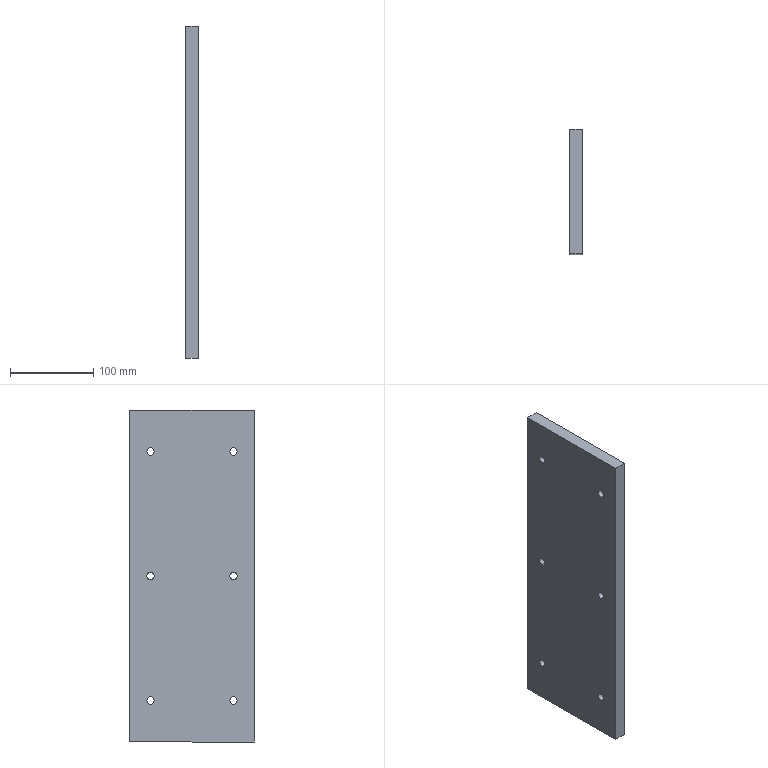Part | SolidWorks | features Extrusion 1, HoleWzd 1 | 1 solid | 36 faces | box 15 x 150 x 400 mm | volume 888167 mm3 | cylinder 24 | plane 12 | commonest cylinder face diameters 9 x12 15 x12
STEP:
#1=CARTESIAN_POINT('',(6.,50.,157.5));
#2=VERTEX_POINT('',#1);
#3=CARTESIAN_POINT('',(6.,50.,142.5));
#4=VERTEX_POINT('',#3);
#5=CARTESIAN_POINT('',(6.,50.,150.));
#6=DIRECTION('',(1.,0.,0.));
#7=DIRECTION('',(0.,0.,-1.));
#8=AXIS2_PLACEMENT_3D('',#5,#6,#7);
#9=CIRCLE('',#8,7.5);
#10=EDGE_CURVE('',#2,#4,#9,.T.);
#11=ORIENTED_EDGE('',*,*,#10,.F.);
#12=CARTESIAN_POINT('',(15.,50.,157.5));
#13=VERTEX_POINT('',#12);
#14=CARTESIAN_POINT('',(15.,50.,157.5));
#15=DIRECTION('',(1.,0.,0.));
#16=VECTOR('',#15,1000.);
#17=LINE('',#14,#16);
#18=EDGE_CURVE('',#2,#13,#17,.T.);
#19=ORIENTED_EDGE('',*,*,#18,.T.);
#20=CARTESIAN_POINT('',(15.,50.,142.5));
#21=VERTEX_POINT('',#20);
#22=CARTESIAN_POINT('',(15.,50.,150.));
#23=DIRECTION('',(1.,0.,0.));
#24=DIRECTION('',(0.,0.,-1.));
#25=AXIS2_PLACEMENT_3D('',#22,#23,#24);
#26=CIRCLE('',#25,7.5);
#27=EDGE_CURVE('',#13,#21,#26,.T.);
#28=ORIENTED_EDGE('',*,*,#27,.T.);
#29=CARTESIAN_POINT('',(15.,50.,142.5));
#30=DIRECTION('',(1.,0.,0.));
#31=VECTOR('',#30,1000.);
#32=LINE('',#29,#31);
#33=EDGE_CURVE('',#4,#21,#32,.T.);
#34=ORIENTED_EDGE('',*,*,#33,.F.);
#35=EDGE_LOOP('',(#11,#19,#28,#34));
#36=FACE_OUTER_BOUND('',#35,.T.);
#37=CARTESIAN_POINT('',(15.,50.,150.));
#38=DIRECTION('',(1.,0.,0.));
#39=DIRECTION('',(0.,0.,-1.));
#40=AXIS2_PLACEMENT_3D('',#37,#38,#39);
#41=CYLINDRICAL_SURFACE('',#40,7.5);
#42=ADVANCED_FACE('',(#36),#41,.F.);
#43=CARTESIAN_POINT('',(0.,50.,154.5));
#44=VERTEX_POINT('',#43);
#45=CARTESIAN_POINT('',(0.,50.,145.5));
#46=VERTEX_POINT('',#45);
#47=CARTESIAN_POINT('',(0.,50.,150.));
#48=DIRECTION('',(1.,0.,0.));
#49=DIRECTION('',(0.,0.,-1.));
#50=AXIS2_PLACEMENT_3D('',#47,#48,#49);
#51=CIRCLE('',#50,4.5);
#52=EDGE_CURVE('',#44,#46,#51,.T.);
#53=ORIENTED_EDGE('',*,*,#52,.F.);
#54=CARTESIAN_POINT('',(6.,50.,154.5));
#55=VERTEX_POINT('',#54);
#56=CARTESIAN_POINT('',(15.,50.,154.5));
#57=DIRECTION('',(1.,0.,0.));
#58=VECTOR('',#57,1000.);
#59=LINE('',#56,#58);
#60=EDGE_CURVE('',#44,#55,#59,.T.);
#61=ORIENTED_EDGE('',*,*,#60,.T.);
#62=CARTESIAN_POINT('',(6.,50.,145.5));
#63=VERTEX_POINT('',#62);
#64=CARTESIAN_POINT('',(6.,50.,150.));
#65=DIRECTION('',(1.,0.,0.));
#66=DIRECTION('',(0.,0.,-1.));
#67=AXIS2_PLACEMENT_3D('',#64,#65,#66);
#68=CIRCLE('',#67,4.5);
#69=EDGE_CURVE('',#55,#63,#68,.T.);
#70=ORIENTED_EDGE('',*,*,#69,.T.);
#71=CARTESIAN_POINT('',(15.,50.,145.5));
#72=DIRECTION('',(1.,0.,0.));
#73=VECTOR('',#72,1000.);
#74=LINE('',#71,#73);
#75=EDGE_CURVE('',#46,#63,#74,.T.);
#76=ORIENTED_EDGE('',*,*,#75,.F.);
#77=EDGE_LOOP('',(#53,#61,#70,#76));
#78=FACE_OUTER_BOUND('',#77,.T.);
#79=CARTESIAN_POINT('',(15.,50.,150.));
#80=DIRECTION('',(1.,0.,0.));
#81=DIRECTION('',(0.,0.,-1.));
#82=AXIS2_PLACEMENT_3D('',#79,#80,#81);
#83=CYLINDRICAL_SURFACE('',#82,4.5);
#84=ADVANCED_FACE('',(#78),#83,.F.);
#85=CARTESIAN_POINT('',(6.,50.,7.5));
#86=VERTEX_POINT('',#85);
#87=CARTESIAN_POINT('',(6.,50.,-7.5));
#88=VERTEX_POINT('',#87);
#89=CARTESIAN_POINT('',(6.,50.,0.));
#90=DIRECTION('',(1.,0.,0.));
#91=DIRECTION('',(0.,0.,-1.));
#92=AXIS2_PLACEMENT_3D('',#89,#90,#91);
#93=CIRCLE('',#92,7.5);
#94=EDGE_CURVE('',#86,#88,#93,.T.);
#95=ORIENTED_EDGE('',*,*,#94,.F.);
#96=CARTESIAN_POINT('',(15.,50.,7.5));
#97=VERTEX_POINT('',#96);
#98=CARTESIAN_POINT('',(15.,50.,7.5));
#99=DIRECTION('',(1.,0.,0.));
#100=VECTOR('',#99,1000.);
#101=LINE('',#98,#100);
#102=EDGE_CURVE('',#86,#97,#101,.T.);
#103=ORIENTED_EDGE('',*,*,#102,.T.);
#104=CARTESIAN_POINT('',(15.,50.,-7.5));
#105=VERTEX_POINT('',#104);
#106=CARTESIAN_POINT('',(15.,50.,0.));
#107=DIRECTION('',(1.,0.,0.));
#108=DIRECTION('',(0.,0.,-1.));
#109=AXIS2_PLACEMENT_3D('',#106,#107,#108);
#110=CIRCLE('',#109,7.5);
#111=EDGE_CURVE('',#97,#105,#110,.T.);
#112=ORIENTED_EDGE('',*,*,#111,.T.);
#113=CARTESIAN_POINT('',(15.,50.,-7.5));
#114=DIRECTION('',(1.,0.,0.));
#115=VECTOR('',#114,1000.);
#116=LINE('',#113,#115);
#117=EDGE_CURVE('',#88,#105,#116,.T.);
#118=ORIENTED_EDGE('',*,*,#117,.F.);
#119=EDGE_LOOP('',(#95,#103,#112,#118));
#120=FACE_OUTER_BOUND('',#119,.T.);
#121=CARTESIAN_POINT('',(15.,50.,0.));
#122=DIRECTION('',(1.,0.,0.));
#123=DIRECTION('',(0.,0.,-1.));
#124=AXIS2_PLACEMENT_3D('',#121,#122,#123);
#125=CYLINDRICAL_SURFACE('',#124,7.5);
#126=ADVANCED_FACE('',(#120),#125,.F.);
#127=CARTESIAN_POINT('',(0.,50.,4.5));
#128=VERTEX_POINT('',#127);
#129=CARTESIAN_POINT('',(0.,50.,-4.5));
#130=VERTEX_POINT('',#129);
#131=CARTESIAN_POINT('',(0.,50.,0.));
#132=DIRECTION('',(1.,0.,0.));
#133=DIRECTION('',(0.,0.,-1.));
#134=AXIS2_PLACEMENT_3D('',#131,#132,#133);
#135=CIRCLE('',#134,4.5);
#136=EDGE_CURVE('',#128,#130,#135,.T.);
#137=ORIENTED_EDGE('',*,*,#136,.F.);
#138=CARTESIAN_POINT('',(6.,50.,4.5));
#139=VERTEX_POINT('',#138);
#140=CARTESIAN_POINT('',(15.,50.,4.5));
#141=DIRECTION('',(1.,0.,0.));
#142=VECTOR('',#141,1000.);
#143=LINE('',#140,#142);
#144=EDGE_CURVE('',#128,#139,#143,.T.);
#145=ORIENTED_EDGE('',*,*,#144,.T.);
#146=CARTESIAN_POINT('',(6.,50.,-4.5));
#147=VERTEX_POINT('',#146);
#148=CARTESIAN_POINT('',(6.,50.,0.));
#149=DIRECTION('',(1.,0.,0.));
#150=DIRECTION('',(0.,0.,-1.));
#151=AXIS2_PLACEMENT_3D('',#148,#149,#150);
#152=CIRCLE('',#151,4.5);
#153=EDGE_CURVE('',#139,#147,#152,.T.);
#154=ORIENTED_EDGE('',*,*,#153,.T.);
#155=CARTESIAN_POINT('',(15.,50.,-4.5));
#156=DIRECTION('',(1.,0.,0.));
#157=VECTOR('',#156,1000.);
#158=LINE('',#155,#157);
#159=EDGE_CURVE('',#130,#147,#158,.T.);
#160=ORIENTED_EDGE('',*,*,#159,.F.);
#161=EDGE_LOOP('',(#137,#145,#154,#160));
#162=FACE_OUTER_BOUND('',#161,.T.);
#163=CARTESIAN_POINT('',(15.,50.,0.));
#164=DIRECTION('',(1.,0.,0.));
#165=DIRECTION('',(0.,0.,-1.));
#166=AXIS2_PLACEMENT_3D('',#163,#164,#165);
#167=CYLINDRICAL_SURFACE('',#166,4.5);
#168=ADVANCED_FACE('',(#162),#167,.F.);
#169=CARTESIAN_POINT('',(6.,50.,-142.5));
#170=VERTEX_POINT('',#169);
#171=CARTESIAN_POINT('',(6.,50.,-157.5));
#172=VERTEX_POINT('',#171);
#173=CARTESIAN_POINT('',(6.,50.,-150.));
#174=DIRECTION('',(1.,0.,0.));
#175=DIRECTION('',(0.,0.,-1.));
#176=AXIS2_PLACEMENT_3D('',#173,#174,#175);
#177=CIRCLE('',#176,7.5);
#178=EDGE_CURVE('',#170,#172,#177,.T.);
#179=ORIENTED_EDGE('',*,*,#178,.F.);
#180=CARTESIAN_POINT('',(15.,50.,-142.5));
#181=VERTEX_POINT('',#180);
#182=CARTESIAN_POINT('',(15.,50.,-142.5));
#183=DIRECTION('',(1.,0.,0.));
#184=VECTOR('',#183,1000.);
#185=LINE('',#182,#184);
#186=EDGE_CURVE('',#170,#181,#185,.T.);
#187=ORIENTED_EDGE('',*,*,#186,.T.);
#188=CARTESIAN_POINT('',(15.,50.,-157.5));
#189=VERTEX_POINT('',#188);
#190=CARTESIAN_POINT('',(15.,50.,-150.));
#191=DIRECTION('',(1.,0.,0.));
#192=DIRECTION('',(0.,0.,-1.));
#193=AXIS2_PLACEMENT_3D('',#190,#191,#192);
#194=CIRCLE('',#193,7.5);
#195=EDGE_CURVE('',#181,#189,#194,.T.);
#196=ORIENTED_EDGE('',*,*,#195,.T.);
#197=CARTESIAN_POINT('',(15.,50.,-157.5));
#198=DIRECTION('',(1.,0.,0.));
#199=VECTOR('',#198,1000.);
#200=LINE('',#197,#199);
#201=EDGE_CURVE('',#172,#189,#200,.T.);
#202=ORIENTED_EDGE('',*,*,#201,.F.);
#203=EDGE_LOOP('',(#179,#187,#196,#202));
#204=FACE_OUTER_BOUND('',#203,.T.);
#205=CARTESIAN_POINT('',(15.,50.,-150.));
#206=DIRECTION('',(1.,0.,0.));
#207=DIRECTION('',(0.,0.,-1.));
#208=AXIS2_PLACEMENT_3D('',#205,#206,#207);
#209=CYLINDRICAL_SURFACE('',#208,7.5);
#210=ADVANCED_FACE('',(#204),#209,.F.);
#211=CARTESIAN_POINT('',(0.,50.,-145.5));
#212=VERTEX_POINT('',#211);
#213=CARTESIAN_POINT('',(0.,50.,-154.5));
#214=VERTEX_POINT('',#213);
#215=CARTESIAN_POINT('',(0.,50.,-150.));
#216=DIRECTION('',(1.,0.,0.));
#217=DIRECTION('',(0.,0.,-1.));
#218=AXIS2_PLACEMENT_3D('',#215,#216,#217);
#219=CIRCLE('',#218,4.5);
#220=EDGE_CURVE('',#212,#214,#219,.T.);
#221=ORIENTED_EDGE('',*,*,#220,.F.);
#222=CARTESIAN_POINT('',(6.,50.,-145.5));
#223=VERTEX_POINT('',#222);
#224=CARTESIAN_POINT('',(15.,50.,-145.5));
#225=DIRECTION('',(1.,0.,0.));
#226=VECTOR('',#225,1000.);
#227=LINE('',#224,#226);
#228=EDGE_CURVE('',#212,#223,#227,.T.);
#229=ORIENTED_EDGE('',*,*,#228,.T.);
#230=CARTESIAN_POINT('',(6.,50.,-154.5));
#231=VERTEX_POINT('',#230);
#232=CARTESIAN_POINT('',(6.,50.,-150.));
#233=DIRECTION('',(1.,0.,0.));
#234=DIRECTION('',(0.,0.,-1.));
#235=AXIS2_PLACEMENT_3D('',#232,#233,#234);
#236=CIRCLE('',#235,4.5);
#237=EDGE_CURVE('',#223,#231,#236,.T.);
#238=ORIENTED_EDGE('',*,*,#237,.T.);
#239=CARTESIAN_POINT('',(15.,50.,-154.5));
#240=DIRECTION('',(1.,0.,0.));
#241=VECTOR('',#240,1000.);
#242=LINE('',#239,#241);
#243=EDGE_CURVE('',#214,#231,#242,.T.);
#244=ORIENTED_EDGE('',*,*,#243,.F.);
#245=EDGE_LOOP('',(#221,#229,#238,#244));
#246=FACE_OUTER_BOUND('',#245,.T.);
#247=CARTESIAN_POINT('',(15.,50.,-150.));
#248=DIRECTION('',(1.,0.,0.));
#249=DIRECTION('',(0.,0.,-1.));
#250=AXIS2_PLACEMENT_3D('',#247,#248,#249);
#251=CYLINDRICAL_SURFACE('',#250,4.5);
#252=ADVANCED_FACE('',(#246),#251,.F.);
#253=CARTESIAN_POINT('',(6.,-50.,157.5));
#254=VERTEX_POINT('',#253);
#255=CARTESIAN_POINT('',(6.,-50.,142.5));
#256=VERTEX_POINT('',#255);
#257=CARTESIAN_POINT('',(6.,-50.,150.));
#258=DIRECTION('',(1.,0.,0.));
#259=DIRECTION('',(0.,0.,-1.));
#260=AXIS2_PLACEMENT_3D('',#257,#258,#259);
#261=CIRCLE('',#260,7.5);
#262=EDGE_CURVE('',#254,#256,#261,.T.);
#263=ORIENTED_EDGE('',*,*,#262,.F.);
#264=CARTESIAN_POINT('',(15.,-50.,157.5));
#265=VERTEX_POINT('',#264);
#266=CARTESIAN_POINT('',(15.,-50.,157.5));
#267=DIRECTION('',(1.,0.,0.));
#268=VECTOR('',#267,1000.);
#269=LINE('',#266,#268);
#270=EDGE_CURVE('',#254,#265,#269,.T.);
#271=ORIENTED_EDGE('',*,*,#270,.T.);
#272=CARTESIAN_POINT('',(15.,-50.,142.5));
#273=VERTEX_POINT('',#272);
#274=CARTESIAN_POINT('',(15.,-50.,150.));
#275=DIRECTION('',(1.,0.,0.));
#276=DIRECTION('',(0.,0.,-1.));
#277=AXIS2_PLACEMENT_3D('',#274,#275,#276);
#278=CIRCLE('',#277,7.5);
#279=EDGE_CURVE('',#265,#273,#278,.T.);
#280=ORIENTED_EDGE('',*,*,#279,.T.);
#281=CARTESIAN_POINT('',(15.,-50.,142.5));
#282=DIRECTION('',(1.,0.,0.));
#283=VECTOR('',#282,1000.);
#284=LINE('',#281,#283);
#285=EDGE_CURVE('',#256,#273,#284,.T.);
#286=ORIENTED_EDGE('',*,*,#285,.F.);
#287=EDGE_LOOP('',(#263,#271,#280,#286));
#288=FACE_OUTER_BOUND('',#287,.T.);
#289=CARTESIAN_POINT('',(15.,-50.,150.));
#290=DIRECTION('',(1.,0.,0.));
#291=DIRECTION('',(0.,0.,-1.));
#292=AXIS2_PLACEMENT_3D('',#289,#290,#291);
#293=CYLINDRICAL_SURFACE('',#292,7.5);
#294=ADVANCED_FACE('',(#288),#293,.F.);
#295=CARTESIAN_POINT('',(0.,-50.,154.5));
#296=VERTEX_POINT('',#295);
#297=CARTESIAN_POINT('',(0.,-50.,145.5));
#298=VERTEX_POINT('',#297);
#299=CARTESIAN_POINT('',(0.,-50.,150.));
#300=DIRECTION('',(1.,0.,0.));
#301=DIRECTION('',(0.,0.,-1.));
#302=AXIS2_PLACEMENT_3D('',#299,#300,#301);
#303=CIRCLE('',#302,4.5);
#304=EDGE_CURVE('',#296,#298,#303,.T.);
#305=ORIENTED_EDGE('',*,*,#304,.F.);
#306=CARTESIAN_POINT('',(6.,-50.,154.5));
#307=VERTEX_POINT('',#306);
#308=CARTESIAN_POINT('',(15.,-50.,154.5));
#309=DIRECTION('',(1.,0.,0.));
#310=VECTOR('',#309,1000.);
#311=LINE('',#308,#310);
#312=EDGE_CURVE('',#296,#307,#311,.T.);
#313=ORIENTED_EDGE('',*,*,#312,.T.);
#314=CARTESIAN_POINT('',(6.,-50.,145.5));
#315=VERTEX_POINT('',#314);
#316=CARTESIAN_POINT('',(6.,-50.,150.));
#317=DIRECTION('',(1.,0.,0.));
#318=DIRECTION('',(0.,0.,-1.));
#319=AXIS2_PLACEMENT_3D('',#316,#317,#318);
#320=CIRCLE('',#319,4.5);
#321=EDGE_CURVE('',#307,#315,#320,.T.);
#322=ORIENTED_EDGE('',*,*,#321,.T.);
#323=CARTESIAN_POINT('',(15.,-50.,145.5));
#324=DIRECTION('',(1.,0.,0.));
#325=VECTOR('',#324,1000.);
#326=LINE('',#323,#325);
#327=EDGE_CURVE('',#298,#315,#326,.T.);
#328=ORIENTED_EDGE('',*,*,#327,.F.);
#329=EDGE_LOOP('',(#305,#313,#322,#328));
#330=FACE_OUTER_BOUND('',#329,.T.);
#331=CARTESIAN_POINT('',(15.,-50.,150.));
#332=DIRECTION('',(1.,0.,0.));
#333=DIRECTION('',(0.,0.,-1.));
#334=AXIS2_PLACEMENT_3D('',#331,#332,#333);
#335=CYLINDRICAL_SURFACE('',#334,4.5);
#336=ADVANCED_FACE('',(#330),#335,.F.);
#337=CARTESIAN_POINT('',(6.,-50.,7.5));
#338=VERTEX_POINT('',#337);
#339=CARTESIAN_POINT('',(6.,-50.,-7.5));
#340=VERTEX_POINT('',#339);
#341=CARTESIAN_POINT('',(6.,-50.,0.));
#342=DIRECTION('',(1.,0.,0.));
#343=DIRECTION('',(0.,0.,-1.));
#344=AXIS2_PLACEMENT_3D('',#341,#342,#343);
#345=CIRCLE('',#344,7.5);
#346=EDGE_CURVE('',#338,#340,#345,.T.);
#347=ORIENTED_EDGE('',*,*,#346,.F.);
#348=CARTESIAN_POINT('',(15.,-50.,7.5));
#349=VERTEX_POINT('',#348);
#350=CARTESIAN_POINT('',(15.,-50.,7.5));
#351=DIRECTION('',(1.,0.,0.));
#352=VECTOR('',#351,1000.);
#353=LINE('',#350,#352);
#354=EDGE_CURVE('',#338,#349,#353,.T.);
#355=ORIENTED_EDGE('',*,*,#354,.T.);
#356=CARTESIAN_POINT('',(15.,-50.,-7.5));
#357=VERTEX_POINT('',#356);
#358=CARTESIAN_POINT('',(15.,-50.,0.));
#359=DIRECTION('',(1.,0.,0.));
#360=DIRECTION('',(0.,0.,-1.));
#361=AXIS2_PLACEMENT_3D('',#358,#359,#360);
#362=CIRCLE('',#361,7.5);
#363=EDGE_CURVE('',#349,#357,#362,.T.);
#364=ORIENTED_EDGE('',*,*,#363,.T.);
#365=CARTESIAN_POINT('',(15.,-50.,-7.5));
#366=DIRECTION('',(1.,0.,0.));
#367=VECTOR('',#366,1000.);
#368=LINE('',#365,#367);
#369=EDGE_CURVE('',#340,#357,#368,.T.);
#370=ORIENTED_EDGE('',*,*,#369,.F.);
#371=EDGE_LOOP('',(#347,#355,#364,#370));
#372=FACE_OUTER_BOUND('',#371,.T.);
#373=CARTESIAN_POINT('',(15.,-50.,0.));
#374=DIRECTION('',(1.,0.,0.));
#375=DIRECTION('',(0.,0.,-1.));
#376=AXIS2_PLACEMENT_3D('',#373,#374,#375);
#377=CYLINDRICAL_SURFACE('',#376,7.5);
#378=ADVANCED_FACE('',(#372),#377,.F.);
#379=CARTESIAN_POINT('',(0.,-50.,4.5));
#380=VERTEX_POINT('',#379);
#381=CARTESIAN_POINT('',(0.,-50.,-4.5));
#382=VERTEX_POINT('',#381);
#383=CARTESIAN_POINT('',(0.,-50.,0.));
#384=DIRECTION('',(1.,0.,0.));
#385=DIRECTION('',(0.,0.,-1.));
#386=AXIS2_PLACEMENT_3D('',#383,#384,#385);
#387=CIRCLE('',#386,4.5);
#388=EDGE_CURVE('',#380,#382,#387,.T.);
#389=ORIENTED_EDGE('',*,*,#388,.F.);
#390=CARTESIAN_POINT('',(6.,-50.,4.5));
#391=VERTEX_POINT('',#390);
#392=CARTESIAN_POINT('',(15.,-50.,4.5));
#393=DIRECTION('',(1.,0.,0.));
#394=VECTOR('',#393,1000.);
#395=LINE('',#392,#394);
#396=EDGE_CURVE('',#380,#391,#395,.T.);
#397=ORIENTED_EDGE('',*,*,#396,.T.);
#398=CARTESIAN_POINT('',(6.,-50.,-4.5));
#399=VERTEX_POINT('',#398);
#400=CARTESIAN_POINT('',(6.,-50.,0.));
#401=DIRECTION('',(1.,0.,0.));
#402=DIRECTION('',(0.,0.,-1.));
#403=AXIS2_PLACEMENT_3D('',#400,#401,#402);
#404=CIRCLE('',#403,4.5);
#405=EDGE_CURVE('',#391,#399,#404,.T.);
#406=ORIENTED_EDGE('',*,*,#405,.T.);
#407=CARTESIAN_POINT('',(15.,-50.,-4.5));
#408=DIRECTION('',(1.,0.,0.));
#409=VECTOR('',#408,1000.);
#410=LINE('',#407,#409);
#411=EDGE_CURVE('',#382,#399,#410,.T.);
#412=ORIENTED_EDGE('',*,*,#411,.F.);
#413=EDGE_LOOP('',(#389,#397,#406,#412));
#414=FACE_OUTER_BOUND('',#413,.T.);
#415=CARTESIAN_POINT('',(15.,-50.,0.));
#416=DIRECTION('',(1.,0.,0.));
#417=DIRECTION('',(0.,0.,-1.));
#418=AXIS2_PLACEMENT_3D('',#415,#416,#417);
#419=CYLINDRICAL_SURFACE('',#418,4.5);
#420=ADVANCED_FACE('',(#414),#419,.F.);
#421=CARTESIAN_POINT('',(6.,-50.,-142.5));
#422=VERTEX_POINT('',#421);
#423=CARTESIAN_POINT('',(6.,-50.,-157.5));
#424=VERTEX_POINT('',#423);
#425=CARTESIAN_POINT('',(6.,-50.,-150.));
#426=DIRECTION('',(1.,0.,0.));
#427=DIRECTION('',(0.,0.,-1.));
#428=AXIS2_PLACEMENT_3D('',#425,#426,#427);
#429=CIRCLE('',#428,7.5);
#430=EDGE_CURVE('',#422,#424,#429,.T.);
#431=ORIENTED_EDGE('',*,*,#430,.F.);
#432=CARTESIAN_POINT('',(15.,-50.,-142.5));
#433=VERTEX_POINT('',#432);
#434=CARTESIAN_POINT('',(15.,-50.,-142.5));
#435=DIRECTION('',(1.,0.,0.));
#436=VECTOR('',#435,1000.);
#437=LINE('',#434,#436);
#438=EDGE_CURVE('',#422,#433,#437,.T.);
#439=ORIENTED_EDGE('',*,*,#438,.T.);
#440=CARTESIAN_POINT('',(15.,-50.,-157.5));
#441=VERTEX_POINT('',#440);
#442=CARTESIAN_POINT('',(15.,-50.,-150.));
#443=DIRECTION('',(1.,0.,0.));
#444=DIRECTION('',(0.,0.,-1.));
#445=AXIS2_PLACEMENT_3D('',#442,#443,#444);
#446=CIRCLE('',#445,7.5);
#447=EDGE_CURVE('',#433,#441,#446,.T.);
#448=ORIENTED_EDGE('',*,*,#447,.T.);
#449=CARTESIAN_POINT('',(15.,-50.,-157.5));
#450=DIRECTION('',(1.,0.,0.));
#451=VECTOR('',#450,1000.);
#452=LINE('',#449,#451);
#453=EDGE_CURVE('',#424,#441,#452,.T.);
#454=ORIENTED_EDGE('',*,*,#453,.F.);
#455=EDGE_LOOP('',(#431,#439,#448,#454));
#456=FACE_OUTER_BOUND('',#455,.T.);
#457=CARTESIAN_POINT('',(15.,-50.,-150.));
#458=DIRECTION('',(1.,0.,0.));
#459=DIRECTION('',(0.,0.,-1.));
#460=AXIS2_PLACEMENT_3D('',#457,#458,#459);
#461=CYLINDRICAL_SURFACE('',#460,7.5);
#462=ADVANCED_FACE('',(#456),#461,.F.);
#463=CARTESIAN_POINT('',(0.,-50.,-145.5));
#464=VERTEX_POINT('',#463);
#465=CARTESIAN_POINT('',(0.,-50.,-154.5));
#466=VERTEX_POINT('',#465);
#467=CARTESIAN_POINT('',(0.,-50.,-150.));
#468=DIRECTION('',(1.,0.,0.));
#469=DIRECTION('',(0.,0.,-1.));
#470=AXIS2_PLACEMENT_3D('',#467,#468,#469);
#471=CIRCLE('',#470,4.5);
#472=EDGE_CURVE('',#464,#466,#471,.T.);
#473=ORIENTED_EDGE('',*,*,#472,.F.);
#474=CARTESIAN_POINT('',(6.,-50.,-145.5));
#475=VERTEX_POINT('',#474);
#476=CARTESIAN_POINT('',(15.,-50.,-145.5));
#477=DIRECTION('',(1.,0.,0.));
#478=VECTOR('',#477,1000.);
#479=LINE('',#476,#478);
#480=EDGE_CURVE('',#464,#475,#479,.T.);
#481=ORIENTED_EDGE('',*,*,#480,.T.);
#482=CARTESIAN_POINT('',(6.,-50.,-154.5));
#483=VERTEX_POINT('',#482);
#484=CARTESIAN_POINT('',(6.,-50.,-150.));
#485=DIRECTION('',(1.,0.,0.));
#486=DIRECTION('',(0.,0.,-1.));
#487=AXIS2_PLACEMENT_3D('',#484,#485,#486);
#488=CIRCLE('',#487,4.5);
#489=EDGE_CURVE('',#475,#483,#488,.T.);
#490=ORIENTED_EDGE('',*,*,#489,.T.);
#491=CARTESIAN_POINT('',(15.,-50.,-154.5));
#492=DIRECTION('',(1.,0.,0.));
#493=VECTOR('',#492,1000.);
#494=LINE('',#491,#493);
#495=EDGE_CURVE('',#466,#483,#494,.T.);
#496=ORIENTED_EDGE('',*,*,#495,.F.);
#497=EDGE_LOOP('',(#473,#481,#490,#496));
#498=FACE_OUTER_BOUND('',#497,.T.);
#499=CARTESIAN_POINT('',(15.,-50.,-150.));
#500=DIRECTION('',(1.,0.,0.));
#501=DIRECTION('',(0.,0.,-1.));
#502=AXIS2_PLACEMENT_3D('',#499,#500,#501);
#503=CYLINDRICAL_SURFACE('',#502,4.5);
#504=ADVANCED_FACE('',(#498),#503,.F.);
#505=CARTESIAN_POINT('',(0.,-75.,-200.));
#506=VERTEX_POINT('',#505);
#507=CARTESIAN_POINT('',(0.,75.,-200.));
#508=VERTEX_POINT('',#507);
#509=CARTESIAN_POINT('',(0.,75.,-200.));
#510=DIRECTION('',(0.,1.,0.));
#511=VECTOR('',#510,1000.);
#512=LINE('',#509,#511);
#513=EDGE_CURVE('',#506,#508,#512,.T.);
#514=ORIENTED_EDGE('',*,*,#513,.T.);
#515=CARTESIAN_POINT('',(15.,75.,-200.));
#516=VERTEX_POINT('',#515);
#517=CARTESIAN_POINT('',(15.,75.,-200.));
#518=DIRECTION('',(-1.,0.,0.));
#519=VECTOR('',#518,1000.);
#520=LINE('',#517,#519);
#521=EDGE_CURVE('',#516,#508,#520,.T.);
#522=ORIENTED_EDGE('',*,*,#521,.F.);
#523=CARTESIAN_POINT('',(15.,-75.,-200.));
#524=VERTEX_POINT('',#523);
#525=CARTESIAN_POINT('',(15.,75.,-200.));
#526=DIRECTION('',(0.,1.,0.));
#527=VECTOR('',#526,1000.);
#528=LINE('',#525,#527);
#529=EDGE_CURVE('',#524,#516,#528,.T.);
#530=ORIENTED_EDGE('',*,*,#529,.F.);
#531=CARTESIAN_POINT('',(15.,-75.,-200.));
#532=DIRECTION('',(-1.,0.,0.));
#533=VECTOR('',#532,1000.);
#534=LINE('',#531,#533);
#535=EDGE_CURVE('',#524,#506,#534,.T.);
#536=ORIENTED_EDGE('',*,*,#535,.T.);
#537=EDGE_LOOP('',(#514,#522,#530,#536));
#538=FACE_OUTER_BOUND('',#537,.T.);
#539=CARTESIAN_POINT('',(15.,75.,-200.));
#540=DIRECTION('',(0.,0.,1.));
#541=DIRECTION('',(0.,-1.,0.));
#542=AXIS2_PLACEMENT_3D('',#539,#540,#541);
#543=PLANE('',#542);
#544=ADVANCED_FACE('',(#538),#543,.F.);
#545=CARTESIAN_POINT('',(0.,75.,200.));
#546=VERTEX_POINT('',#545);
#547=CARTESIAN_POINT('',(0.,75.,200.));
#548=DIRECTION('',(0.,0.,1.));
#549=VECTOR('',#548,1000.);
#550=LINE('',#547,#549);
#551=EDGE_CURVE('',#508,#546,#550,.T.);
#552=ORIENTED_EDGE('',*,*,#551,.T.);
#553=CARTESIAN_POINT('',(15.,75.,200.));
#554=VERTEX_POINT('',#553);
#555=CARTESIAN_POINT('',(15.,75.,200.));
#556=DIRECTION('',(-1.,0.,0.));
#557=VECTOR('',#556,1000.);
#558=LINE('',#555,#557);
#559=EDGE_CURVE('',#554,#546,#558,.T.);
#560=ORIENTED_EDGE('',*,*,#559,.F.);
#561=CARTESIAN_POINT('',(15.,75.,200.));
#562=DIRECTION('',(0.,0.,1.));
#563=VECTOR('',#562,1000.);
#564=LINE('',#561,#563);
#565=EDGE_CURVE('',#516,#554,#564,.T.);
#566=ORIENTED_EDGE('',*,*,#565,.F.);
#567=ORIENTED_EDGE('',*,*,#521,.T.);
#568=EDGE_LOOP('',(#552,#560,#566,#567));
#569=FACE_OUTER_BOUND('',#568,.T.);
#570=CARTESIAN_POINT('',(15.,75.,200.));
#571=DIRECTION('',(0.,-1.,0.));
#572=DIRECTION('',(0.,0.,-1.));
#573=AXIS2_PLACEMENT_3D('',#570,#571,#572);
#574=PLANE('',#573);
#575=ADVANCED_FACE('',(#569),#574,.F.);
#576=CARTESIAN_POINT('',(0.,-75.,200.));
#577=VERTEX_POINT('',#576);
#578=CARTESIAN_POINT('',(0.,75.,200.));
#579=DIRECTION('',(0.,-1.,0.));
#580=VECTOR('',#579,1000.);
#581=LINE('',#578,#580);
#582=EDGE_CURVE('',#546,#577,#581,.T.);
#583=ORIENTED_EDGE('',*,*,#582,.T.);
#584=CARTESIAN_POINT('',(15.,-75.,200.));
#585=VERTEX_POINT('',#584);
#586=CARTESIAN_POINT('',(15.,-75.,200.));
#587=DIRECTION('',(-1.,0.,0.));
#588=VECTOR('',#587,1000.);
#589=LINE('',#586,#588);
#590=EDGE_CURVE('',#585,#577,#589,.T.);
#591=ORIENTED_EDGE('',*,*,#590,.F.);
#592=CARTESIAN_POINT('',(15.,75.,200.));
#593=DIRECTION('',(0.,-1.,0.));
#594=VECTOR('',#593,1000.);
#595=LINE('',#592,#594);
#596=EDGE_CURVE('',#554,#585,#595,.T.);
#597=ORIENTED_EDGE('',*,*,#596,.F.);
#598=ORIENTED_EDGE('',*,*,#559,.T.);
#599=EDGE_LOOP('',(#583,#591,#597,#598));
#600=FACE_OUTER_BOUND('',#599,.T.);
#601=CARTESIAN_POINT('',(15.,75.,200.));
#602=DIRECTION('',(0.,0.,-1.));
#603=DIRECTION('',(0.,1.,0.));
#604=AXIS2_PLACEMENT_3D('',#601,#602,#603);
#605=PLANE('',#604);
#606=ADVANCED_FACE('',(#600),#605,.F.);
#607=CARTESIAN_POINT('',(0.,-75.,200.));
#608=DIRECTION('',(0.,0.,-1.));
#609=VECTOR('',#608,1000.);
#610=LINE('',#607,#609);
#611=EDGE_CURVE('',#577,#506,#610,.T.);
#612=ORIENTED_EDGE('',*,*,#611,.T.);
#613=ORIENTED_EDGE('',*,*,#535,.F.);
#614=CARTESIAN_POINT('',(15.,-75.,200.));
#615=DIRECTION('',(0.,0.,-1.));
#616=VECTOR('',#615,1000.);
#617=LINE('',#614,#616);
#618=EDGE_CURVE('',#585,#524,#617,.T.);
#619=ORIENTED_EDGE('',*,*,#618,.F.);
#620=ORIENTED_EDGE('',*,*,#590,.T.);
#621=EDGE_LOOP('',(#612,#613,#619,#620));
#622=FACE_OUTER_BOUND('',#621,.T.);
#623=CARTESIAN_POINT('',(15.,-75.,200.));
#624=DIRECTION('',(0.,1.,0.));
#625=DIRECTION('',(0.,0.,1.));
#626=AXIS2_PLACEMENT_3D('',#623,#624,#625);
#627=PLANE('',#626);
#628=ADVANCED_FACE('',(#622),#627,.F.);
#629=CARTESIAN_POINT('',(15.,50.,150.));
#630=DIRECTION('',(1.,0.,0.));
#631=DIRECTION('',(0.,0.,-1.));
#632=AXIS2_PLACEMENT_3D('',#629,#630,#631);
#633=CIRCLE('',#632,7.5);
#634=EDGE_CURVE('',#21,#13,#633,.T.);
#635=ORIENTED_EDGE('',*,*,#634,.F.);
#636=ORIENTED_EDGE('',*,*,#27,.F.);
#637=EDGE_LOOP('',(#635,#636));
#638=FACE_BOUND('',#637,.T.);
#639=CARTESIAN_POINT('',(15.,50.,0.));
#640=DIRECTION('',(1.,0.,0.));
#641=DIRECTION('',(0.,0.,-1.));
#642=AXIS2_PLACEMENT_3D('',#639,#640,#641);
#643=CIRCLE('',#642,7.5);
#644=EDGE_CURVE('',#105,#97,#643,.T.);
#645=ORIENTED_EDGE('',*,*,#644,.F.);
#646=ORIENTED_EDGE('',*,*,#111,.F.);
#647=EDGE_LOOP('',(#645,#646));
#648=FACE_BOUND('',#647,.T.);
#649=CARTESIAN_POINT('',(15.,50.,-150.));
#650=DIRECTION('',(1.,0.,0.));
#651=DIRECTION('',(0.,0.,-1.));
#652=AXIS2_PLACEMENT_3D('',#649,#650,#651);
#653=CIRCLE('',#652,7.5);
#654=EDGE_CURVE('',#189,#181,#653,.T.);
#655=ORIENTED_EDGE('',*,*,#654,.F.);
#656=ORIENTED_EDGE('',*,*,#195,.F.);
#657=EDGE_LOOP('',(#655,#656));
#658=FACE_BOUND('',#657,.T.);
#659=CARTESIAN_POINT('',(15.,-50.,150.));
#660=DIRECTION('',(1.,0.,0.));
#661=DIRECTION('',(0.,0.,-1.));
#662=AXIS2_PLACEMENT_3D('',#659,#660,#661);
#663=CIRCLE('',#662,7.5);
#664=EDGE_CURVE('',#273,#265,#663,.T.);
#665=ORIENTED_EDGE('',*,*,#664,.F.);
#666=ORIENTED_EDGE('',*,*,#279,.F.);
#667=EDGE_LOOP('',(#665,#666));
#668=FACE_BOUND('',#667,.T.);
#669=CARTESIAN_POINT('',(15.,-50.,0.));
#670=DIRECTION('',(1.,0.,0.));
#671=DIRECTION('',(0.,0.,-1.));
#672=AXIS2_PLACEMENT_3D('',#669,#670,#671);
#673=CIRCLE('',#672,7.5);
#674=EDGE_CURVE('',#357,#349,#673,.T.);
#675=ORIENTED_EDGE('',*,*,#674,.F.);
#676=ORIENTED_EDGE('',*,*,#363,.F.);
#677=EDGE_LOOP('',(#675,#676));
#678=FACE_BOUND('',#677,.T.);
#679=CARTESIAN_POINT('',(15.,-50.,-150.));
#680=DIRECTION('',(1.,0.,0.));
#681=DIRECTION('',(0.,0.,-1.));
#682=AXIS2_PLACEMENT_3D('',#679,#680,#681);
#683=CIRCLE('',#682,7.5);
#684=EDGE_CURVE('',#441,#433,#683,.T.);
#685=ORIENTED_EDGE('',*,*,#684,.F.);
#686=ORIENTED_EDGE('',*,*,#447,.F.);
#687=EDGE_LOOP('',(#685,#686));
#688=FACE_BOUND('',#687,.T.);
#689=ORIENTED_EDGE('',*,*,#529,.T.);
#690=ORIENTED_EDGE('',*,*,#565,.T.);
#691=ORIENTED_EDGE('',*,*,#596,.T.);
#692=ORIENTED_EDGE('',*,*,#618,.T.);
#693=EDGE_LOOP('',(#689,#690,#691,#692));
#694=FACE_OUTER_BOUND('',#693,.T.);
#695=CARTESIAN_POINT('',(15.,0.,0.));
#696=DIRECTION('',(1.,0.,0.));
#697=DIRECTION('',(0.,0.,-1.));
#698=AXIS2_PLACEMENT_3D('',#695,#696,#697);
#699=PLANE('',#698);
#700=ADVANCED_FACE('',(#638,#648,#658,#668,#678,#688,#694),#699,.T.);
#701=CARTESIAN_POINT('',(0.,50.,150.));
#702=DIRECTION('',(1.,0.,0.));
#703=DIRECTION('',(0.,0.,-1.));
#704=AXIS2_PLACEMENT_3D('',#701,#702,#703);
#705=CIRCLE('',#704,4.5);
#706=EDGE_CURVE('',#46,#44,#705,.T.);
#707=ORIENTED_EDGE('',*,*,#706,.T.);
#708=ORIENTED_EDGE('',*,*,#52,.T.);
#709=EDGE_LOOP('',(#707,#708));
#710=FACE_BOUND('',#709,.T.);
#711=CARTESIAN_POINT('',(0.,50.,0.));
#712=DIRECTION('',(1.,0.,0.));
#713=DIRECTION('',(0.,0.,-1.));
#714=AXIS2_PLACEMENT_3D('',#711,#712,#713);
#715=CIRCLE('',#714,4.5);
#716=EDGE_CURVE('',#130,#128,#715,.T.);
#717=ORIENTED_EDGE('',*,*,#716,.T.);
#718=ORIENTED_EDGE('',*,*,#136,.T.);
#719=EDGE_LOOP('',(#717,#718));
#720=FACE_BOUND('',#719,.T.);
#721=CARTESIAN_POINT('',(0.,50.,-150.));
#722=DIRECTION('',(1.,0.,0.));
#723=DIRECTION('',(0.,0.,-1.));
#724=AXIS2_PLACEMENT_3D('',#721,#722,#723);
#725=CIRCLE('',#724,4.5);
#726=EDGE_CURVE('',#214,#212,#725,.T.);
#727=ORIENTED_EDGE('',*,*,#726,.T.);
#728=ORIENTED_EDGE('',*,*,#220,.T.);
#729=EDGE_LOOP('',(#727,#728));
#730=FACE_BOUND('',#729,.T.);
#731=CARTESIAN_POINT('',(0.,-50.,150.));
#732=DIRECTION('',(1.,0.,0.));
#733=DIRECTION('',(0.,0.,-1.));
#734=AXIS2_PLACEMENT_3D('',#731,#732,#733);
#735=CIRCLE('',#734,4.5);
#736=EDGE_CURVE('',#298,#296,#735,.T.);
#737=ORIENTED_EDGE('',*,*,#736,.T.);
#738=ORIENTED_EDGE('',*,*,#304,.T.);
#739=EDGE_LOOP('',(#737,#738));
#740=FACE_BOUND('',#739,.T.);
#741=CARTESIAN_POINT('',(0.,-50.,0.));
#742=DIRECTION('',(1.,0.,0.));
#743=DIRECTION('',(0.,0.,-1.));
#744=AXIS2_PLACEMENT_3D('',#741,#742,#743);
#745=CIRCLE('',#744,4.5);
#746=EDGE_CURVE('',#382,#380,#745,.T.);
#747=ORIENTED_EDGE('',*,*,#746,.T.);
#748=ORIENTED_EDGE('',*,*,#388,.T.);
#749=EDGE_LOOP('',(#747,#748));
#750=FACE_BOUND('',#749,.T.);
#751=CARTESIAN_POINT('',(0.,-50.,-150.));
#752=DIRECTION('',(1.,0.,0.));
#753=DIRECTION('',(0.,0.,-1.));
#754=AXIS2_PLACEMENT_3D('',#751,#752,#753);
#755=CIRCLE('',#754,4.5);
#756=EDGE_CURVE('',#466,#464,#755,.T.);
#757=ORIENTED_EDGE('',*,*,#756,.T.);
#758=ORIENTED_EDGE('',*,*,#472,.T.);
#759=EDGE_LOOP('',(#757,#758));
#760=FACE_BOUND('',#759,.T.);
#761=ORIENTED_EDGE('',*,*,#513,.F.);
#762=ORIENTED_EDGE('',*,*,#611,.F.);
#763=ORIENTED_EDGE('',*,*,#582,.F.);
#764=ORIENTED_EDGE('',*,*,#551,.F.);
#765=EDGE_LOOP('',(#761,#762,#763,#764));
#766=FACE_OUTER_BOUND('',#765,.T.);
#767=CARTESIAN_POINT('',(0.,0.,0.));
#768=DIRECTION('',(1.,0.,0.));
#769=DIRECTION('',(0.,0.,-1.));
#770=AXIS2_PLACEMENT_3D('',#767,#768,#769);
#771=PLANE('',#770);
#772=ADVANCED_FACE('',(#710,#720,#730,#740,#750,#760,#766),#771,.F.);
#773=ORIENTED_EDGE('',*,*,#480,.F.);
#774=ORIENTED_EDGE('',*,*,#756,.F.);
#775=ORIENTED_EDGE('',*,*,#495,.T.);
#776=CARTESIAN_POINT('',(6.,-50.,-150.));
#777=DIRECTION('',(1.,0.,0.));
#778=DIRECTION('',(0.,0.,-1.));
#779=AXIS2_PLACEMENT_3D('',#776,#777,#778);
#780=CIRCLE('',#779,4.5);
#781=EDGE_CURVE('',#483,#475,#780,.T.);
#782=ORIENTED_EDGE('',*,*,#781,.T.);
#783=EDGE_LOOP('',(#773,#774,#775,#782));
#784=FACE_OUTER_BOUND('',#783,.T.);
#785=CARTESIAN_POINT('',(15.,-50.,-150.));
#786=DIRECTION('',(1.,0.,0.));
#787=DIRECTION('',(0.,0.,-1.));
#788=AXIS2_PLACEMENT_3D('',#785,#786,#787);
#789=CYLINDRICAL_SURFACE('',#788,4.5);
#790=ADVANCED_FACE('',(#784),#789,.F.);
#791=ORIENTED_EDGE('',*,*,#781,.F.);
#792=ORIENTED_EDGE('',*,*,#489,.F.);
#793=EDGE_LOOP('',(#791,#792));
#794=FACE_BOUND('',#793,.T.);
#795=CARTESIAN_POINT('',(6.,-50.,-150.));
#796=DIRECTION('',(1.,0.,0.));
#797=DIRECTION('',(0.,0.,-1.));
#798=AXIS2_PLACEMENT_3D('',#795,#796,#797);
#799=CIRCLE('',#798,7.5);
#800=EDGE_CURVE('',#424,#422,#799,.T.);
#801=ORIENTED_EDGE('',*,*,#800,.T.);
#802=ORIENTED_EDGE('',*,*,#430,.T.);
#803=EDGE_LOOP('',(#801,#802));
#804=FACE_OUTER_BOUND('',#803,.T.);
#805=CARTESIAN_POINT('',(6.,-45.5,-150.));
#806=DIRECTION('',(-1.,0.,0.));
#807=DIRECTION('',(0.,0.,1.));
#808=AXIS2_PLACEMENT_3D('',#805,#806,#807);
#809=PLANE('',#808);
#810=ADVANCED_FACE('',(#794,#804),#809,.F.);
#811=ORIENTED_EDGE('',*,*,#438,.F.);
#812=ORIENTED_EDGE('',*,*,#800,.F.);
#813=ORIENTED_EDGE('',*,*,#453,.T.);
#814=ORIENTED_EDGE('',*,*,#684,.T.);
#815=EDGE_LOOP('',(#811,#812,#813,#814));
#816=FACE_OUTER_BOUND('',#815,.T.);
#817=CARTESIAN_POINT('',(15.,-50.,-150.));
#818=DIRECTION('',(1.,0.,0.));
#819=DIRECTION('',(0.,0.,-1.));
#820=AXIS2_PLACEMENT_3D('',#817,#818,#819);
#821=CYLINDRICAL_SURFACE('',#820,7.5);
#822=ADVANCED_FACE('',(#816),#821,.F.);
#823=ORIENTED_EDGE('',*,*,#396,.F.);
#824=ORIENTED_EDGE('',*,*,#746,.F.);
#825=ORIENTED_EDGE('',*,*,#411,.T.);
#826=CARTESIAN_POINT('',(6.,-50.,0.));
#827=DIRECTION('',(1.,0.,0.));
#828=DIRECTION('',(0.,0.,-1.));
#829=AXIS2_PLACEMENT_3D('',#826,#827,#828);
#830=CIRCLE('',#829,4.5);
#831=EDGE_CURVE('',#399,#391,#830,.T.);
#832=ORIENTED_EDGE('',*,*,#831,.T.);
#833=EDGE_LOOP('',(#823,#824,#825,#832));
#834=FACE_OUTER_BOUND('',#833,.T.);
#835=CARTESIAN_POINT('',(15.,-50.,0.));
#836=DIRECTION('',(1.,0.,0.));
#837=DIRECTION('',(0.,0.,-1.));
#838=AXIS2_PLACEMENT_3D('',#835,#836,#837);
#839=CYLINDRICAL_SURFACE('',#838,4.5);
#840=ADVANCED_FACE('',(#834),#839,.F.);
#841=ORIENTED_EDGE('',*,*,#831,.F.);
#842=ORIENTED_EDGE('',*,*,#405,.F.);
#843=EDGE_LOOP('',(#841,#842));
#844=FACE_BOUND('',#843,.T.);
#845=CARTESIAN_POINT('',(6.,-50.,0.));
#846=DIRECTION('',(1.,0.,0.));
#847=DIRECTION('',(0.,0.,-1.));
#848=AXIS2_PLACEMENT_3D('',#845,#846,#847);
#849=CIRCLE('',#848,7.5);
#850=EDGE_CURVE('',#340,#338,#849,.T.);
#851=ORIENTED_EDGE('',*,*,#850,.T.);
#852=ORIENTED_EDGE('',*,*,#346,.T.);
#853=EDGE_LOOP('',(#851,#852));
#854=FACE_OUTER_BOUND('',#853,.T.);
#855=CARTESIAN_POINT('',(6.,-45.5,0.));
#856=DIRECTION('',(-1.,0.,0.));
#857=DIRECTION('',(0.,0.,1.));
#858=AXIS2_PLACEMENT_3D('',#855,#856,#857);
#859=PLANE('',#858);
#860=ADVANCED_FACE('',(#844,#854),#859,.F.);
#861=ORIENTED_EDGE('',*,*,#354,.F.);
#862=ORIENTED_EDGE('',*,*,#850,.F.);
#863=ORIENTED_EDGE('',*,*,#369,.T.);
#864=ORIENTED_EDGE('',*,*,#674,.T.);
#865=EDGE_LOOP('',(#861,#862,#863,#864));
#866=FACE_OUTER_BOUND('',#865,.T.);
#867=CARTESIAN_POINT('',(15.,-50.,0.));
#868=DIRECTION('',(1.,0.,0.));
#869=DIRECTION('',(0.,0.,-1.));
#870=AXIS2_PLACEMENT_3D('',#867,#868,#869);
#871=CYLINDRICAL_SURFACE('',#870,7.5);
#872=ADVANCED_FACE('',(#866),#871,.F.);
#873=ORIENTED_EDGE('',*,*,#312,.F.);
#874=ORIENTED_EDGE('',*,*,#736,.F.);
#875=ORIENTED_EDGE('',*,*,#327,.T.);
#876=CARTESIAN_POINT('',(6.,-50.,150.));
#877=DIRECTION('',(1.,0.,0.));
#878=DIRECTION('',(0.,0.,-1.));
#879=AXIS2_PLACEMENT_3D('',#876,#877,#878);
#880=CIRCLE('',#879,4.5);
#881=EDGE_CURVE('',#315,#307,#880,.T.);
#882=ORIENTED_EDGE('',*,*,#881,.T.);
#883=EDGE_LOOP('',(#873,#874,#875,#882));
#884=FACE_OUTER_BOUND('',#883,.T.);
#885=CARTESIAN_POINT('',(15.,-50.,150.));
#886=DIRECTION('',(1.,0.,0.));
#887=DIRECTION('',(0.,0.,-1.));
#888=AXIS2_PLACEMENT_3D('',#885,#886,#887);
#889=CYLINDRICAL_SURFACE('',#888,4.5);
#890=ADVANCED_FACE('',(#884),#889,.F.);
#891=ORIENTED_EDGE('',*,*,#881,.F.);
#892=ORIENTED_EDGE('',*,*,#321,.F.);
#893=EDGE_LOOP('',(#891,#892));
#894=FACE_BOUND('',#893,.T.);
#895=CARTESIAN_POINT('',(6.,-50.,150.));
#896=DIRECTION('',(1.,0.,0.));
#897=DIRECTION('',(0.,0.,-1.));
#898=AXIS2_PLACEMENT_3D('',#895,#896,#897);
#899=CIRCLE('',#898,7.5);
#900=EDGE_CURVE('',#256,#254,#899,.T.);
#901=ORIENTED_EDGE('',*,*,#900,.T.);
#902=ORIENTED_EDGE('',*,*,#262,.T.);
#903=EDGE_LOOP('',(#901,#902));
#904=FACE_OUTER_BOUND('',#903,.T.);
#905=CARTESIAN_POINT('',(6.,-45.5,150.));
#906=DIRECTION('',(-1.,0.,0.));
#907=DIRECTION('',(0.,0.,1.));
#908=AXIS2_PLACEMENT_3D('',#905,#906,#907);
#909=PLANE('',#908);
#910=ADVANCED_FACE('',(#894,#904),#909,.F.);
#911=ORIENTED_EDGE('',*,*,#270,.F.);
#912=ORIENTED_EDGE('',*,*,#900,.F.);
#913=ORIENTED_EDGE('',*,*,#285,.T.);
#914=ORIENTED_EDGE('',*,*,#664,.T.);
#915=EDGE_LOOP('',(#911,#912,#913,#914));
#916=FACE_OUTER_BOUND('',#915,.T.);
#917=CARTESIAN_POINT('',(15.,-50.,150.));
#918=DIRECTION('',(1.,0.,0.));
#919=DIRECTION('',(0.,0.,-1.));
#920=AXIS2_PLACEMENT_3D('',#917,#918,#919);
#921=CYLINDRICAL_SURFACE('',#920,7.5);
#922=ADVANCED_FACE('',(#916),#921,.F.);
#923=ORIENTED_EDGE('',*,*,#228,.F.);
#924=ORIENTED_EDGE('',*,*,#726,.F.);
#925=ORIENTED_EDGE('',*,*,#243,.T.);
#926=CARTESIAN_POINT('',(6.,50.,-150.));
#927=DIRECTION('',(1.,0.,0.));
#928=DIRECTION('',(0.,0.,-1.));
#929=AXIS2_PLACEMENT_3D('',#926,#927,#928);
#930=CIRCLE('',#929,4.5);
#931=EDGE_CURVE('',#231,#223,#930,.T.);
#932=ORIENTED_EDGE('',*,*,#931,.T.);
#933=EDGE_LOOP('',(#923,#924,#925,#932));
#934=FACE_OUTER_BOUND('',#933,.T.);
#935=CARTESIAN_POINT('',(15.,50.,-150.));
#936=DIRECTION('',(1.,0.,0.));
#937=DIRECTION('',(0.,0.,-1.));
#938=AXIS2_PLACEMENT_3D('',#935,#936,#937);
#939=CYLINDRICAL_SURFACE('',#938,4.5);
#940=ADVANCED_FACE('',(#934),#939,.F.);
#941=ORIENTED_EDGE('',*,*,#931,.F.);
#942=ORIENTED_EDGE('',*,*,#237,.F.);
#943=EDGE_LOOP('',(#941,#942));
#944=FACE_BOUND('',#943,.T.);
#945=CARTESIAN_POINT('',(6.,50.,-150.));
#946=DIRECTION('',(1.,0.,0.));
#947=DIRECTION('',(0.,0.,-1.));
#948=AXIS2_PLACEMENT_3D('',#945,#946,#947);
#949=CIRCLE('',#948,7.5);
#950=EDGE_CURVE('',#172,#170,#949,.T.);
#951=ORIENTED_EDGE('',*,*,#950,.T.);
#952=ORIENTED_EDGE('',*,*,#178,.T.);
#953=EDGE_LOOP('',(#951,#952));
#954=FACE_OUTER_BOUND('',#953,.T.);
#955=CARTESIAN_POINT('',(6.,54.5,-150.));
#956=DIRECTION('',(-1.,0.,0.));
#957=DIRECTION('',(0.,0.,1.));
#958=AXIS2_PLACEMENT_3D('',#955,#956,#957);
#959=PLANE('',#958);
#960=ADVANCED_FACE('',(#944,#954),#959,.F.);
#961=ORIENTED_EDGE('',*,*,#186,.F.);
#962=ORIENTED_EDGE('',*,*,#950,.F.);
#963=ORIENTED_EDGE('',*,*,#201,.T.);
#964=ORIENTED_EDGE('',*,*,#654,.T.);
#965=EDGE_LOOP('',(#961,#962,#963,#964));
#966=FACE_OUTER_BOUND('',#965,.T.);
#967=CARTESIAN_POINT('',(15.,50.,-150.));
#968=DIRECTION('',(1.,0.,0.));
#969=DIRECTION('',(0.,0.,-1.));
#970=AXIS2_PLACEMENT_3D('',#967,#968,#969);
#971=CYLINDRICAL_SURFACE('',#970,7.5);
#972=ADVANCED_FACE('',(#966),#971,.F.);
#973=ORIENTED_EDGE('',*,*,#144,.F.);
#974=ORIENTED_EDGE('',*,*,#716,.F.);
#975=ORIENTED_EDGE('',*,*,#159,.T.);
#976=CARTESIAN_POINT('',(6.,50.,0.));
#977=DIRECTION('',(1.,0.,0.));
#978=DIRECTION('',(0.,0.,-1.));
#979=AXIS2_PLACEMENT_3D('',#976,#977,#978);
#980=CIRCLE('',#979,4.5);
#981=EDGE_CURVE('',#147,#139,#980,.T.);
#982=ORIENTED_EDGE('',*,*,#981,.T.);
#983=EDGE_LOOP('',(#973,#974,#975,#982));
#984=FACE_OUTER_BOUND('',#983,.T.);
#985=CARTESIAN_POINT('',(15.,50.,0.));
#986=DIRECTION('',(1.,0.,0.));
#987=DIRECTION('',(0.,0.,-1.));
#988=AXIS2_PLACEMENT_3D('',#985,#986,#987);
#989=CYLINDRICAL_SURFACE('',#988,4.5);
#990=ADVANCED_FACE('',(#984),#989,.F.);
#991=ORIENTED_EDGE('',*,*,#981,.F.);
#992=ORIENTED_EDGE('',*,*,#153,.F.);
#993=EDGE_LOOP('',(#991,#992));
#994=FACE_BOUND('',#993,.T.);
#995=CARTESIAN_POINT('',(6.,50.,0.));
#996=DIRECTION('',(1.,0.,0.));
#997=DIRECTION('',(0.,0.,-1.));
#998=AXIS2_PLACEMENT_3D('',#995,#996,#997);
#999=CIRCLE('',#998,7.5);
#1000=EDGE_CURVE('',#88,#86,#999,.T.);
#1001=ORIENTED_EDGE('',*,*,#1000,.T.);
#1002=ORIENTED_EDGE('',*,*,#94,.T.);
#1003=EDGE_LOOP('',(#1001,#1002));
#1004=FACE_OUTER_BOUND('',#1003,.T.);
#1005=CARTESIAN_POINT('',(6.,54.5,0.));
#1006=DIRECTION('',(-1.,0.,0.));
#1007=DIRECTION('',(0.,0.,1.));
#1008=AXIS2_PLACEMENT_3D('',#1005,#1006,#1007);
#1009=PLANE('',#1008);
#1010=ADVANCED_FACE('',(#994,#1004),#1009,.F.);
#1011=ORIENTED_EDGE('',*,*,#102,.F.);
#1012=ORIENTED_EDGE('',*,*,#1000,.F.);
#1013=ORIENTED_EDGE('',*,*,#117,.T.);
#1014=ORIENTED_EDGE('',*,*,#644,.T.);
#1015=EDGE_LOOP('',(#1011,#1012,#1013,#1014));
#1016=FACE_OUTER_BOUND('',#1015,.T.);
#1017=CARTESIAN_POINT('',(15.,50.,0.));
#1018=DIRECTION('',(1.,0.,0.));
#1019=DIRECTION('',(0.,0.,-1.));
#1020=AXIS2_PLACEMENT_3D('',#1017,#1018,#1019);
#1021=CYLINDRICAL_SURFACE('',#1020,7.5);
#1022=ADVANCED_FACE('',(#1016),#1021,.F.);
#1023=ORIENTED_EDGE('',*,*,#60,.F.);
#1024=ORIENTED_EDGE('',*,*,#706,.F.);
#1025=ORIENTED_EDGE('',*,*,#75,.T.);
#1026=CARTESIAN_POINT('',(6.,50.,150.));
#1027=DIRECTION('',(1.,0.,0.));
#1028=DIRECTION('',(0.,0.,-1.));
#1029=AXIS2_PLACEMENT_3D('',#1026,#1027,#1028);
#1030=CIRCLE('',#1029,4.5);
#1031=EDGE_CURVE('',#63,#55,#1030,.T.);
#1032=ORIENTED_EDGE('',*,*,#1031,.T.);
#1033=EDGE_LOOP('',(#1023,#1024,#1025,#1032));
#1034=FACE_OUTER_BOUND('',#1033,.T.);
#1035=CARTESIAN_POINT('',(15.,50.,150.));
#1036=DIRECTION('',(1.,0.,0.));
#1037=DIRECTION('',(0.,0.,-1.));
#1038=AXIS2_PLACEMENT_3D('',#1035,#1036,#1037);
#1039=CYLINDRICAL_SURFACE('',#1038,4.5);
#1040=ADVANCED_FACE('',(#1034),#1039,.F.);
#1041=ORIENTED_EDGE('',*,*,#1031,.F.);
#1042=ORIENTED_EDGE('',*,*,#69,.F.);
#1043=EDGE_LOOP('',(#1041,#1042));
#1044=FACE_BOUND('',#1043,.T.);
#1045=CARTESIAN_POINT('',(6.,50.,150.));
#1046=DIRECTION('',(1.,0.,0.));
#1047=DIRECTION('',(0.,0.,-1.));
#1048=AXIS2_PLACEMENT_3D('',#1045,#1046,#1047);
#1049=CIRCLE('',#1048,7.5);
#1050=EDGE_CURVE('',#4,#2,#1049,.T.);
#1051=ORIENTED_EDGE('',*,*,#1050,.T.);
#1052=ORIENTED_EDGE('',*,*,#10,.T.);
#1053=EDGE_LOOP('',(#1051,#1052));
#1054=FACE_OUTER_BOUND('',#1053,.T.);
#1055=CARTESIAN_POINT('',(6.,54.5,150.));
#1056=DIRECTION('',(-1.,0.,0.));
#1057=DIRECTION('',(0.,0.,1.));
#1058=AXIS2_PLACEMENT_3D('',#1055,#1056,#1057);
#1059=PLANE('',#1058);
#1060=ADVANCED_FACE('',(#1044,#1054),#1059,.F.);
#1061=ORIENTED_EDGE('',*,*,#18,.F.);
#1062=ORIENTED_EDGE('',*,*,#1050,.F.);
#1063=ORIENTED_EDGE('',*,*,#33,.T.);
#1064=ORIENTED_EDGE('',*,*,#634,.T.);
#1065=EDGE_LOOP('',(#1061,#1062,#1063,#1064));
#1066=FACE_OUTER_BOUND('',#1065,.T.);
#1067=CARTESIAN_POINT('',(15.,50.,150.));
#1068=DIRECTION('',(1.,0.,0.));
#1069=DIRECTION('',(0.,0.,-1.));
#1070=AXIS2_PLACEMENT_3D('',#1067,#1068,#1069);
#1071=CYLINDRICAL_SURFACE('',#1070,7.5);
#1072=ADVANCED_FACE('',(#1066),#1071,.F.);
#1073=CLOSED_SHELL('',(#42,#84,#126,#168,#210,#252,#294,#336,#378,#420,#462,#504,#544,#575,#606,#628,#700,#772,#790,#810,#822,#840,#860,#872,#890,#910,#922,#940,#960,#972,#990,#1010,#1022,#1040,#1060,#1072));
#1074=MANIFOLD_SOLID_BREP('',#1073);
#1075=CARTESIAN_POINT('',(0.,0.,0.));
#1076=DIRECTION('',(0.,0.,1.));
#1077=DIRECTION('',(1.,0.,0.));
#1078=AXIS2_PLACEMENT_3D('',#1075,#1076,#1077);
#1079=(LENGTH_UNIT()NAMED_UNIT(*)SI_UNIT(.MILLI.,.METRE.));
#1080=UNCERTAINTY_MEASURE_WITH_UNIT(LENGTH_MEASURE(0.00001),#1079,'','');
#1081=(NAMED_UNIT(*)PLANE_ANGLE_UNIT()SI_UNIT($,.RADIAN.));
#1082=(NAMED_UNIT(*)SI_UNIT($,.STERADIAN.)SOLID_ANGLE_UNIT());
#1083=(GEOMETRIC_REPRESENTATION_CONTEXT(3)GLOBAL_UNCERTAINTY_ASSIGNED_CONTEXT((#1080))GLOBAL_UNIT_ASSIGNED_CONTEXT((#1079,#1081,#1082))REPRESENTATION_CONTEXT('',''));
#1084=ADVANCED_BREP_SHAPE_REPRESENTATION('',(#1074,#1078),#1083);